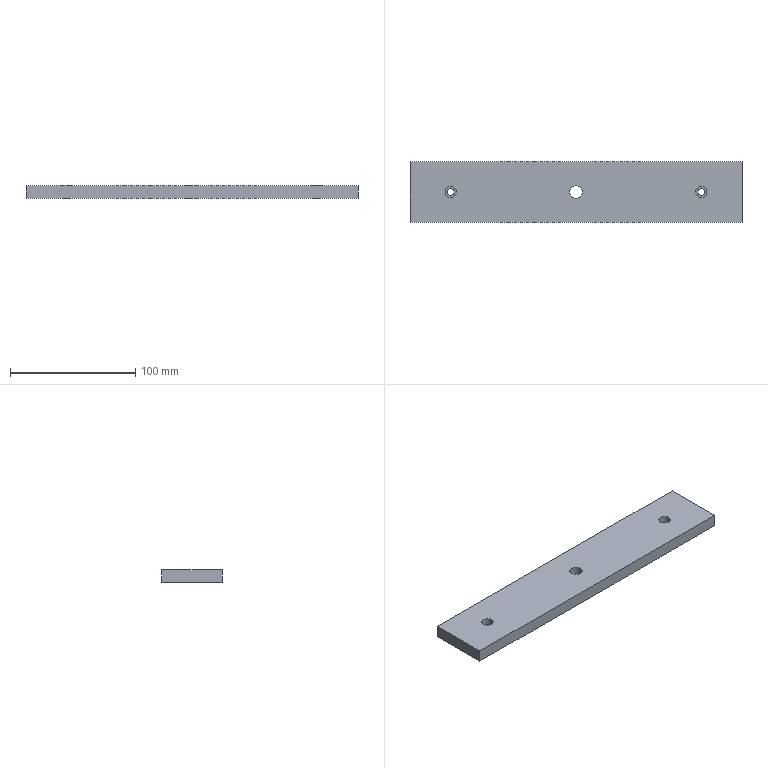Part | STEP file | B1-008 | 1 solid | 18 faces | box 265 x 48 x 10 mm | volume 125461 mm3 | cylinder 10 | plane 8 | commonest cylinder face diameters 5.5 x4 9 x4 10 x2
STEP:
#1=CARTESIAN_POINT('',(0.,0.,0.));
#2=DIRECTION('',(0.,0.,1.));
#3=DIRECTION('',(1.,0.,0.));
#4=AXIS2_PLACEMENT_3D('',#1,#2,#3);
#5=CARTESIAN_POINT('',(-95.5,0.,-1.));
#6=VERTEX_POINT('',#5);
#7=CARTESIAN_POINT('',(-95.5,0.,5.));
#8=VERTEX_POINT('',#7);
#9=CARTESIAN_POINT('',(-95.5,0.,-1.));
#10=DIRECTION('',(0.,0.,1.));
#11=VECTOR('',#10,1.);
#12=LINE('',#9,#11);
#13=CARTESIAN_POINT('',(-100.,0.,-1.));
#14=DIRECTION('',(0.,0.,1.));
#15=DIRECTION('',(1.,0.,0.));
#16=AXIS2_PLACEMENT_3D('',#13,#14,#15);
#17=CYLINDRICAL_SURFACE('',#16,4.5);
#18=CARTESIAN_POINT('',(6.283,0.));
#19=DIRECTION('',(0.,1.));
#20=VECTOR('',#19,1.);
#21=LINE('',#18,#20);
#22=(GEOMETRIC_REPRESENTATION_CONTEXT(2)PARAMETRIC_REPRESENTATION_CONTEXT()REPRESENTATION_CONTEXT('',''));
#23=DEFINITIONAL_REPRESENTATION('',(#21),#22);
#24=PCURVE('',#17,#23);
#25=CARTESIAN_POINT('',(-100.,0.,-1.));
#26=DIRECTION('',(0.,0.,1.));
#27=DIRECTION('',(1.,0.,0.));
#28=AXIS2_PLACEMENT_3D('',#25,#26,#27);
#29=CYLINDRICAL_SURFACE('',#28,4.5);
#30=CARTESIAN_POINT('',(0.,0.));
#31=DIRECTION('',(0.,1.));
#32=VECTOR('',#31,1.);
#33=LINE('',#30,#32);
#34=(GEOMETRIC_REPRESENTATION_CONTEXT(2)PARAMETRIC_REPRESENTATION_CONTEXT()REPRESENTATION_CONTEXT('',''));
#35=DEFINITIONAL_REPRESENTATION('',(#33),#34);
#36=PCURVE('',#29,#35);
#37=SURFACE_CURVE('',#12,(#24,#36),.PCURVE_S1.);
#38=EDGE_CURVE('',#6,#8,#37,.T.);
#39=ORIENTED_EDGE('',*,*,#38,.T.);
#40=CARTESIAN_POINT('',(-104.5,0.,5.));
#41=VERTEX_POINT('',#40);
#42=CARTESIAN_POINT('',(-100.,0.,5.));
#43=DIRECTION('',(0.,0.,1.));
#44=DIRECTION('',(1.,0.,0.));
#45=AXIS2_PLACEMENT_3D('',#42,#43,#44);
#46=CIRCLE('',#45,4.5);
#47=CARTESIAN_POINT('',(0.,6.));
#48=DIRECTION('',(1.,0.));
#49=VECTOR('',#48,1.);
#50=LINE('',#47,#49);
#51=(GEOMETRIC_REPRESENTATION_CONTEXT(2)PARAMETRIC_REPRESENTATION_CONTEXT()REPRESENTATION_CONTEXT('',''));
#52=DEFINITIONAL_REPRESENTATION('',(#50),#51);
#53=PCURVE('',#17,#52);
#54=CARTESIAN_POINT('',(0.,0.,5.));
#55=DIRECTION('',(0.,0.,1.));
#56=DIRECTION('',(1.,0.,0.));
#57=AXIS2_PLACEMENT_3D('',#54,#55,#56);
#58=PLANE('',#57);
#59=CARTESIAN_POINT('',(-100.,0.));
#60=DIRECTION('',(1.,0.));
#61=AXIS2_PLACEMENT_2D('',#59,#60);
#62=CIRCLE('',#61,4.5);
#63=(GEOMETRIC_REPRESENTATION_CONTEXT(2)PARAMETRIC_REPRESENTATION_CONTEXT()REPRESENTATION_CONTEXT('',''));
#64=DEFINITIONAL_REPRESENTATION('',(#62),#63);
#65=PCURVE('',#58,#64);
#66=SURFACE_CURVE('',#46,(#53,#65),.PCURVE_S1.);
#67=EDGE_CURVE('',#41,#8,#66,.T.);
#68=ORIENTED_EDGE('',*,*,#67,.F.);
#69=CARTESIAN_POINT('',(-104.5,0.,-1.));
#70=VERTEX_POINT('',#69);
#71=CARTESIAN_POINT('',(-104.5,0.,-1.));
#72=DIRECTION('',(0.,0.,1.));
#73=VECTOR('',#72,1.);
#74=LINE('',#71,#73);
#75=CARTESIAN_POINT('',(3.142,0.));
#76=DIRECTION('',(0.,1.));
#77=VECTOR('',#76,1.);
#78=LINE('',#75,#77);
#79=(GEOMETRIC_REPRESENTATION_CONTEXT(2)PARAMETRIC_REPRESENTATION_CONTEXT()REPRESENTATION_CONTEXT('',''));
#80=DEFINITIONAL_REPRESENTATION('',(#78),#79);
#81=PCURVE('',#17,#80);
#82=CARTESIAN_POINT('',(3.142,0.));
#83=DIRECTION('',(0.,1.));
#84=VECTOR('',#83,1.);
#85=LINE('',#82,#84);
#86=(GEOMETRIC_REPRESENTATION_CONTEXT(2)PARAMETRIC_REPRESENTATION_CONTEXT()REPRESENTATION_CONTEXT('',''));
#87=DEFINITIONAL_REPRESENTATION('',(#85),#86);
#88=PCURVE('',#29,#87);
#89=SURFACE_CURVE('',#74,(#81,#88),.PCURVE_S1.);
#90=EDGE_CURVE('',#70,#41,#89,.T.);
#91=ORIENTED_EDGE('',*,*,#90,.F.);
#92=CARTESIAN_POINT('',(-100.,0.,-1.));
#93=DIRECTION('',(0.,0.,1.));
#94=DIRECTION('',(1.,0.,0.));
#95=AXIS2_PLACEMENT_3D('',#92,#93,#94);
#96=CIRCLE('',#95,4.5);
#97=CARTESIAN_POINT('',(0.,0.));
#98=DIRECTION('',(1.,0.));
#99=VECTOR('',#98,1.);
#100=LINE('',#97,#99);
#101=(GEOMETRIC_REPRESENTATION_CONTEXT(2)PARAMETRIC_REPRESENTATION_CONTEXT()REPRESENTATION_CONTEXT('',''));
#102=DEFINITIONAL_REPRESENTATION('',(#100),#101);
#103=PCURVE('',#17,#102);
#104=CARTESIAN_POINT('',(-100.,0.,-1.));
#105=DIRECTION('',(0.,0.,1.));
#106=DIRECTION('',(1.,0.,0.));
#107=AXIS2_PLACEMENT_3D('',#104,#105,#106);
#108=PLANE('',#107);
#109=CARTESIAN_POINT('',(0.,0.));
#110=DIRECTION('',(1.,0.));
#111=AXIS2_PLACEMENT_2D('',#109,#110);
#112=CIRCLE('',#111,4.5);
#113=(GEOMETRIC_REPRESENTATION_CONTEXT(2)PARAMETRIC_REPRESENTATION_CONTEXT()REPRESENTATION_CONTEXT('',''));
#114=DEFINITIONAL_REPRESENTATION('',(#112),#113);
#115=PCURVE('',#108,#114);
#116=SURFACE_CURVE('',#96,(#103,#115),.PCURVE_S1.);
#117=EDGE_CURVE('',#70,#6,#116,.T.);
#118=ORIENTED_EDGE('',*,*,#117,.T.);
#119=EDGE_LOOP('',(#39,#68,#91,#118));
#120=FACE_BOUND('',#119,.F.);
#121=ADVANCED_FACE('',(#120),#17,.F.);
#122=CARTESIAN_POINT('',(104.5,0.,-1.));
#123=VERTEX_POINT('',#122);
#124=CARTESIAN_POINT('',(104.5,0.,5.));
#125=VERTEX_POINT('',#124);
#126=CARTESIAN_POINT('',(104.5,0.,-1.));
#127=DIRECTION('',(0.,0.,1.));
#128=VECTOR('',#127,1.);
#129=LINE('',#126,#128);
#130=CARTESIAN_POINT('',(100.,0.,-1.));
#131=DIRECTION('',(0.,0.,1.));
#132=DIRECTION('',(1.,0.,0.));
#133=AXIS2_PLACEMENT_3D('',#130,#131,#132);
#134=CYLINDRICAL_SURFACE('',#133,4.5);
#135=CARTESIAN_POINT('',(6.283,0.));
#136=DIRECTION('',(0.,1.));
#137=VECTOR('',#136,1.);
#138=LINE('',#135,#137);
#139=(GEOMETRIC_REPRESENTATION_CONTEXT(2)PARAMETRIC_REPRESENTATION_CONTEXT()REPRESENTATION_CONTEXT('',''));
#140=DEFINITIONAL_REPRESENTATION('',(#138),#139);
#141=PCURVE('',#134,#140);
#142=CARTESIAN_POINT('',(100.,0.,-1.));
#143=DIRECTION('',(0.,0.,1.));
#144=DIRECTION('',(1.,0.,0.));
#145=AXIS2_PLACEMENT_3D('',#142,#143,#144);
#146=CYLINDRICAL_SURFACE('',#145,4.5);
#147=CARTESIAN_POINT('',(0.,0.));
#148=DIRECTION('',(0.,1.));
#149=VECTOR('',#148,1.);
#150=LINE('',#147,#149);
#151=(GEOMETRIC_REPRESENTATION_CONTEXT(2)PARAMETRIC_REPRESENTATION_CONTEXT()REPRESENTATION_CONTEXT('',''));
#152=DEFINITIONAL_REPRESENTATION('',(#150),#151);
#153=PCURVE('',#146,#152);
#154=SURFACE_CURVE('',#129,(#141,#153),.PCURVE_S1.);
#155=EDGE_CURVE('',#123,#125,#154,.T.);
#156=ORIENTED_EDGE('',*,*,#155,.T.);
#157=CARTESIAN_POINT('',(95.5,0.,5.));
#158=VERTEX_POINT('',#157);
#159=CARTESIAN_POINT('',(100.,0.,5.));
#160=DIRECTION('',(0.,0.,1.));
#161=DIRECTION('',(1.,0.,0.));
#162=AXIS2_PLACEMENT_3D('',#159,#160,#161);
#163=CIRCLE('',#162,4.5);
#164=CARTESIAN_POINT('',(0.,6.));
#165=DIRECTION('',(1.,0.));
#166=VECTOR('',#165,1.);
#167=LINE('',#164,#166);
#168=(GEOMETRIC_REPRESENTATION_CONTEXT(2)PARAMETRIC_REPRESENTATION_CONTEXT()REPRESENTATION_CONTEXT('',''));
#169=DEFINITIONAL_REPRESENTATION('',(#167),#168);
#170=PCURVE('',#134,#169);
#171=CARTESIAN_POINT('',(100.,0.));
#172=DIRECTION('',(1.,0.));
#173=AXIS2_PLACEMENT_2D('',#171,#172);
#174=CIRCLE('',#173,4.5);
#175=(GEOMETRIC_REPRESENTATION_CONTEXT(2)PARAMETRIC_REPRESENTATION_CONTEXT()REPRESENTATION_CONTEXT('',''));
#176=DEFINITIONAL_REPRESENTATION('',(#174),#175);
#177=PCURVE('',#58,#176);
#178=SURFACE_CURVE('',#163,(#170,#177),.PCURVE_S1.);
#179=EDGE_CURVE('',#158,#125,#178,.T.);
#180=ORIENTED_EDGE('',*,*,#179,.F.);
#181=CARTESIAN_POINT('',(95.5,0.,-1.));
#182=VERTEX_POINT('',#181);
#183=CARTESIAN_POINT('',(95.5,0.,-1.));
#184=DIRECTION('',(0.,0.,1.));
#185=VECTOR('',#184,1.);
#186=LINE('',#183,#185);
#187=CARTESIAN_POINT('',(3.142,0.));
#188=DIRECTION('',(0.,1.));
#189=VECTOR('',#188,1.);
#190=LINE('',#187,#189);
#191=(GEOMETRIC_REPRESENTATION_CONTEXT(2)PARAMETRIC_REPRESENTATION_CONTEXT()REPRESENTATION_CONTEXT('',''));
#192=DEFINITIONAL_REPRESENTATION('',(#190),#191);
#193=PCURVE('',#134,#192);
#194=CARTESIAN_POINT('',(3.142,0.));
#195=DIRECTION('',(0.,1.));
#196=VECTOR('',#195,1.);
#197=LINE('',#194,#196);
#198=(GEOMETRIC_REPRESENTATION_CONTEXT(2)PARAMETRIC_REPRESENTATION_CONTEXT()REPRESENTATION_CONTEXT('',''));
#199=DEFINITIONAL_REPRESENTATION('',(#197),#198);
#200=PCURVE('',#146,#199);
#201=SURFACE_CURVE('',#186,(#193,#200),.PCURVE_S1.);
#202=EDGE_CURVE('',#182,#158,#201,.T.);
#203=ORIENTED_EDGE('',*,*,#202,.F.);
#204=CARTESIAN_POINT('',(100.,0.,-1.));
#205=DIRECTION('',(0.,0.,1.));
#206=DIRECTION('',(1.,0.,0.));
#207=AXIS2_PLACEMENT_3D('',#204,#205,#206);
#208=CIRCLE('',#207,4.5);
#209=CARTESIAN_POINT('',(0.,0.));
#210=DIRECTION('',(1.,0.));
#211=VECTOR('',#210,1.);
#212=LINE('',#209,#211);
#213=(GEOMETRIC_REPRESENTATION_CONTEXT(2)PARAMETRIC_REPRESENTATION_CONTEXT()REPRESENTATION_CONTEXT('',''));
#214=DEFINITIONAL_REPRESENTATION('',(#212),#213);
#215=PCURVE('',#134,#214);
#216=CARTESIAN_POINT('',(100.,0.,-1.));
#217=DIRECTION('',(0.,0.,1.));
#218=DIRECTION('',(1.,0.,0.));
#219=AXIS2_PLACEMENT_3D('',#216,#217,#218);
#220=PLANE('',#219);
#221=CARTESIAN_POINT('',(0.,0.));
#222=DIRECTION('',(1.,0.));
#223=AXIS2_PLACEMENT_2D('',#221,#222);
#224=CIRCLE('',#223,4.5);
#225=(GEOMETRIC_REPRESENTATION_CONTEXT(2)PARAMETRIC_REPRESENTATION_CONTEXT()REPRESENTATION_CONTEXT('',''));
#226=DEFINITIONAL_REPRESENTATION('',(#224),#225);
#227=PCURVE('',#220,#226);
#228=SURFACE_CURVE('',#208,(#215,#227),.PCURVE_S1.);
#229=EDGE_CURVE('',#182,#123,#228,.T.);
#230=ORIENTED_EDGE('',*,*,#229,.T.);
#231=EDGE_LOOP('',(#156,#180,#203,#230));
#232=FACE_BOUND('',#231,.F.);
#233=ADVANCED_FACE('',(#232),#134,.F.);
#234=CARTESIAN_POINT('',(5.,0.,-5.));
#235=VERTEX_POINT('',#234);
#236=CARTESIAN_POINT('',(5.,0.,5.));
#237=VERTEX_POINT('',#236);
#238=CARTESIAN_POINT('',(5.,0.,-19.142));
#239=DIRECTION('',(0.,0.,1.));
#240=VECTOR('',#239,1.);
#241=LINE('',#238,#240);
#242=CARTESIAN_POINT('',(0.,0.,-19.142));
#243=DIRECTION('',(0.,0.,1.));
#244=DIRECTION('',(1.,0.,0.));
#245=AXIS2_PLACEMENT_3D('',#242,#243,#244);
#246=CYLINDRICAL_SURFACE('',#245,5.);
#247=CARTESIAN_POINT('',(6.283,0.));
#248=DIRECTION('',(0.,1.));
#249=VECTOR('',#248,1.);
#250=LINE('',#247,#249);
#251=(GEOMETRIC_REPRESENTATION_CONTEXT(2)PARAMETRIC_REPRESENTATION_CONTEXT()REPRESENTATION_CONTEXT('',''));
#252=DEFINITIONAL_REPRESENTATION('',(#250),#251);
#253=PCURVE('',#246,#252);
#254=CARTESIAN_POINT('',(0.,0.,-19.142));
#255=DIRECTION('',(0.,0.,1.));
#256=DIRECTION('',(1.,0.,0.));
#257=AXIS2_PLACEMENT_3D('',#254,#255,#256);
#258=CYLINDRICAL_SURFACE('',#257,5.);
#259=CARTESIAN_POINT('',(0.,0.));
#260=DIRECTION('',(0.,1.));
#261=VECTOR('',#260,1.);
#262=LINE('',#259,#261);
#263=(GEOMETRIC_REPRESENTATION_CONTEXT(2)PARAMETRIC_REPRESENTATION_CONTEXT()REPRESENTATION_CONTEXT('',''));
#264=DEFINITIONAL_REPRESENTATION('',(#262),#263);
#265=PCURVE('',#258,#264);
#266=SURFACE_CURVE('',#241,(#253,#265),.PCURVE_S1.);
#267=EDGE_CURVE('',#235,#237,#266,.T.);
#268=ORIENTED_EDGE('',*,*,#267,.T.);
#269=CARTESIAN_POINT('',(-5.,0.,5.));
#270=VERTEX_POINT('',#269);
#271=CARTESIAN_POINT('',(0.,0.,5.));
#272=DIRECTION('',(0.,0.,1.));
#273=DIRECTION('',(1.,0.,0.));
#274=AXIS2_PLACEMENT_3D('',#271,#272,#273);
#275=CIRCLE('',#274,5.);
#276=CARTESIAN_POINT('',(0.,24.142));
#277=DIRECTION('',(1.,0.));
#278=VECTOR('',#277,1.);
#279=LINE('',#276,#278);
#280=(GEOMETRIC_REPRESENTATION_CONTEXT(2)PARAMETRIC_REPRESENTATION_CONTEXT()REPRESENTATION_CONTEXT('',''));
#281=DEFINITIONAL_REPRESENTATION('',(#279),#280);
#282=PCURVE('',#246,#281);
#283=CARTESIAN_POINT('',(0.,0.));
#284=DIRECTION('',(1.,0.));
#285=AXIS2_PLACEMENT_2D('',#283,#284);
#286=CIRCLE('',#285,5.);
#287=(GEOMETRIC_REPRESENTATION_CONTEXT(2)PARAMETRIC_REPRESENTATION_CONTEXT()REPRESENTATION_CONTEXT('',''));
#288=DEFINITIONAL_REPRESENTATION('',(#286),#287);
#289=PCURVE('',#58,#288);
#290=SURFACE_CURVE('',#275,(#282,#289),.PCURVE_S1.);
#291=EDGE_CURVE('',#270,#237,#290,.T.);
#292=ORIENTED_EDGE('',*,*,#291,.F.);
#293=CARTESIAN_POINT('',(-5.,0.,-5.));
#294=VERTEX_POINT('',#293);
#295=CARTESIAN_POINT('',(-5.,0.,-19.142));
#296=DIRECTION('',(0.,0.,1.));
#297=VECTOR('',#296,1.);
#298=LINE('',#295,#297);
#299=CARTESIAN_POINT('',(3.142,0.));
#300=DIRECTION('',(0.,1.));
#301=VECTOR('',#300,1.);
#302=LINE('',#299,#301);
#303=(GEOMETRIC_REPRESENTATION_CONTEXT(2)PARAMETRIC_REPRESENTATION_CONTEXT()REPRESENTATION_CONTEXT('',''));
#304=DEFINITIONAL_REPRESENTATION('',(#302),#303);
#305=PCURVE('',#246,#304);
#306=CARTESIAN_POINT('',(3.142,0.));
#307=DIRECTION('',(0.,1.));
#308=VECTOR('',#307,1.);
#309=LINE('',#306,#308);
#310=(GEOMETRIC_REPRESENTATION_CONTEXT(2)PARAMETRIC_REPRESENTATION_CONTEXT()REPRESENTATION_CONTEXT('',''));
#311=DEFINITIONAL_REPRESENTATION('',(#309),#310);
#312=PCURVE('',#258,#311);
#313=SURFACE_CURVE('',#298,(#305,#312),.PCURVE_S1.);
#314=EDGE_CURVE('',#294,#270,#313,.T.);
#315=ORIENTED_EDGE('',*,*,#314,.F.);
#316=CARTESIAN_POINT('',(0.,0.,-5.));
#317=DIRECTION('',(0.,0.,-1.));
#318=DIRECTION('',(1.,0.,0.));
#319=AXIS2_PLACEMENT_3D('',#316,#317,#318);
#320=CIRCLE('',#319,5.);
#321=CARTESIAN_POINT('',(6.283,14.142));
#322=DIRECTION('',(-1.,0.));
#323=VECTOR('',#322,1.);
#324=LINE('',#321,#323);
#325=(GEOMETRIC_REPRESENTATION_CONTEXT(2)PARAMETRIC_REPRESENTATION_CONTEXT()REPRESENTATION_CONTEXT('',''));
#326=DEFINITIONAL_REPRESENTATION('',(#324),#325);
#327=PCURVE('',#246,#326);
#328=CARTESIAN_POINT('',(0.,0.,-5.));
#329=DIRECTION('',(0.,0.,1.));
#330=DIRECTION('',(1.,0.,0.));
#331=AXIS2_PLACEMENT_3D('',#328,#329,#330);
#332=PLANE('',#331);
#333=CARTESIAN_POINT('',(5.,0.));
#334=CARTESIAN_POINT('',(5.,-8.66));
#335=CARTESIAN_POINT('',(-2.5,-4.33));
#336=CARTESIAN_POINT('',(-10.,0.));
#337=CARTESIAN_POINT('',(-2.5,4.33));
#338=CARTESIAN_POINT('',(5.,8.66));
#339=CARTESIAN_POINT('',(5.,0.));
#340=(BOUNDED_CURVE()B_SPLINE_CURVE(2,(#333,#334,#335,#336,#337,#338,#339),.UNSPECIFIED.,.T.,.F.)B_SPLINE_CURVE_WITH_KNOTS((1,2,2,2,2,1),(-2.094,0.,2.094,4.189,6.283,8.378),.UNSPECIFIED.)CURVE()GEOMETRIC_REPRESENTATION_ITEM()RATIONAL_B_SPLINE_CURVE((1.,0.5,1.,0.5,1.,0.5,1.))REPRESENTATION_ITEM(''));
#341=(GEOMETRIC_REPRESENTATION_CONTEXT(2)PARAMETRIC_REPRESENTATION_CONTEXT()REPRESENTATION_CONTEXT('',''));
#342=DEFINITIONAL_REPRESENTATION('',(#340),#341);
#343=PCURVE('',#332,#342);
#344=SURFACE_CURVE('',#320,(#327,#343),.PCURVE_S1.);
#345=EDGE_CURVE('',#235,#294,#344,.T.);
#346=ORIENTED_EDGE('',*,*,#345,.F.);
#347=EDGE_LOOP('',(#268,#292,#315,#346));
#348=FACE_BOUND('',#347,.F.);
#349=ADVANCED_FACE('',(#348),#246,.F.);
#350=CARTESIAN_POINT('',(97.25,0.,-1.));
#351=VERTEX_POINT('',#350);
#352=CARTESIAN_POINT('',(97.25,0.,-5.));
#353=VERTEX_POINT('',#352);
#354=CARTESIAN_POINT('',(97.25,0.,12.778));
#355=DIRECTION('',(0.,0.,-1.));
#356=VECTOR('',#355,1.);
#357=LINE('',#354,#356);
#358=CARTESIAN_POINT('',(100.,0.,12.778));
#359=DIRECTION('',(0.,0.,-1.));
#360=DIRECTION('',(-1.,0.,0.));
#361=AXIS2_PLACEMENT_3D('',#358,#359,#360);
#362=CYLINDRICAL_SURFACE('',#361,2.75);
#363=CARTESIAN_POINT('',(6.283,0.));
#364=DIRECTION('',(0.,1.));
#365=VECTOR('',#364,1.);
#366=LINE('',#363,#365);
#367=(GEOMETRIC_REPRESENTATION_CONTEXT(2)PARAMETRIC_REPRESENTATION_CONTEXT()REPRESENTATION_CONTEXT('',''));
#368=DEFINITIONAL_REPRESENTATION('',(#366),#367);
#369=PCURVE('',#362,#368);
#370=CARTESIAN_POINT('',(100.,0.,12.778));
#371=DIRECTION('',(0.,0.,-1.));
#372=DIRECTION('',(-1.,0.,0.));
#373=AXIS2_PLACEMENT_3D('',#370,#371,#372);
#374=CYLINDRICAL_SURFACE('',#373,2.75);
#375=CARTESIAN_POINT('',(0.,0.));
#376=DIRECTION('',(0.,1.));
#377=VECTOR('',#376,1.);
#378=LINE('',#375,#377);
#379=(GEOMETRIC_REPRESENTATION_CONTEXT(2)PARAMETRIC_REPRESENTATION_CONTEXT()REPRESENTATION_CONTEXT('',''));
#380=DEFINITIONAL_REPRESENTATION('',(#378),#379);
#381=PCURVE('',#374,#380);
#382=SURFACE_CURVE('',#357,(#369,#381),.PCURVE_S1.);
#383=EDGE_CURVE('',#351,#353,#382,.T.);
#384=ORIENTED_EDGE('',*,*,#383,.T.);
#385=CARTESIAN_POINT('',(102.75,0.,-5.));
#386=VERTEX_POINT('',#385);
#387=CARTESIAN_POINT('',(100.,0.,-5.));
#388=DIRECTION('',(0.,0.,-1.));
#389=DIRECTION('',(-1.,0.,0.));
#390=AXIS2_PLACEMENT_3D('',#387,#388,#389);
#391=CIRCLE('',#390,2.75);
#392=CARTESIAN_POINT('',(0.,17.778));
#393=DIRECTION('',(1.,0.));
#394=VECTOR('',#393,1.);
#395=LINE('',#392,#394);
#396=(GEOMETRIC_REPRESENTATION_CONTEXT(2)PARAMETRIC_REPRESENTATION_CONTEXT()REPRESENTATION_CONTEXT('',''));
#397=DEFINITIONAL_REPRESENTATION('',(#395),#396);
#398=PCURVE('',#362,#397);
#399=CARTESIAN_POINT('',(97.25,0.));
#400=CARTESIAN_POINT('',(97.25,4.763));
#401=CARTESIAN_POINT('',(101.375,2.382));
#402=CARTESIAN_POINT('',(105.5,0.));
#403=CARTESIAN_POINT('',(101.375,-2.382));
#404=CARTESIAN_POINT('',(97.25,-4.763));
#405=CARTESIAN_POINT('',(97.25,0.));
#406=(BOUNDED_CURVE()B_SPLINE_CURVE(2,(#399,#400,#401,#402,#403,#404,#405),.UNSPECIFIED.,.T.,.F.)B_SPLINE_CURVE_WITH_KNOTS((1,2,2,2,2,1),(-2.094,0.,2.094,4.189,6.283,8.378),.UNSPECIFIED.)CURVE()GEOMETRIC_REPRESENTATION_ITEM()RATIONAL_B_SPLINE_CURVE((1.,0.5,1.,0.5,1.,0.5,1.))REPRESENTATION_ITEM(''));
#407=(GEOMETRIC_REPRESENTATION_CONTEXT(2)PARAMETRIC_REPRESENTATION_CONTEXT()REPRESENTATION_CONTEXT('',''));
#408=DEFINITIONAL_REPRESENTATION('',(#406),#407);
#409=PCURVE('',#332,#408);
#410=SURFACE_CURVE('',#391,(#398,#409),.PCURVE_S1.);
#411=EDGE_CURVE('',#386,#353,#410,.T.);
#412=ORIENTED_EDGE('',*,*,#411,.F.);
#413=CARTESIAN_POINT('',(102.75,0.,-1.));
#414=VERTEX_POINT('',#413);
#415=CARTESIAN_POINT('',(102.75,0.,12.778));
#416=DIRECTION('',(0.,0.,-1.));
#417=VECTOR('',#416,1.);
#418=LINE('',#415,#417);
#419=CARTESIAN_POINT('',(3.142,0.));
#420=DIRECTION('',(0.,1.));
#421=VECTOR('',#420,1.);
#422=LINE('',#419,#421);
#423=(GEOMETRIC_REPRESENTATION_CONTEXT(2)PARAMETRIC_REPRESENTATION_CONTEXT()REPRESENTATION_CONTEXT('',''));
#424=DEFINITIONAL_REPRESENTATION('',(#422),#423);
#425=PCURVE('',#362,#424);
#426=CARTESIAN_POINT('',(3.142,0.));
#427=DIRECTION('',(0.,1.));
#428=VECTOR('',#427,1.);
#429=LINE('',#426,#428);
#430=(GEOMETRIC_REPRESENTATION_CONTEXT(2)PARAMETRIC_REPRESENTATION_CONTEXT()REPRESENTATION_CONTEXT('',''));
#431=DEFINITIONAL_REPRESENTATION('',(#429),#430);
#432=PCURVE('',#374,#431);
#433=SURFACE_CURVE('',#418,(#425,#432),.PCURVE_S1.);
#434=EDGE_CURVE('',#414,#386,#433,.T.);
#435=ORIENTED_EDGE('',*,*,#434,.F.);
#436=CARTESIAN_POINT('',(100.,0.,-1.));
#437=DIRECTION('',(0.,0.,-1.));
#438=DIRECTION('',(1.,0.,0.));
#439=AXIS2_PLACEMENT_3D('',#436,#437,#438);
#440=CIRCLE('',#439,2.75);
#441=CARTESIAN_POINT('',(3.142,13.778));
#442=DIRECTION('',(1.,0.));
#443=VECTOR('',#442,1.);
#444=LINE('',#441,#443);
#445=(GEOMETRIC_REPRESENTATION_CONTEXT(2)PARAMETRIC_REPRESENTATION_CONTEXT()REPRESENTATION_CONTEXT('',''));
#446=DEFINITIONAL_REPRESENTATION('',(#444),#445);
#447=PCURVE('',#362,#446);
#448=CARTESIAN_POINT('',(2.75,0.));
#449=CARTESIAN_POINT('',(2.75,-4.763));
#450=CARTESIAN_POINT('',(-1.375,-2.382));
#451=CARTESIAN_POINT('',(-5.5,0.));
#452=CARTESIAN_POINT('',(-1.375,2.382));
#453=CARTESIAN_POINT('',(2.75,4.763));
#454=CARTESIAN_POINT('',(2.75,0.));
#455=(BOUNDED_CURVE()B_SPLINE_CURVE(2,(#448,#449,#450,#451,#452,#453,#454),.UNSPECIFIED.,.T.,.F.)B_SPLINE_CURVE_WITH_KNOTS((1,2,2,2,2,1),(-2.094,0.,2.094,4.189,6.283,8.378),.UNSPECIFIED.)CURVE()GEOMETRIC_REPRESENTATION_ITEM()RATIONAL_B_SPLINE_CURVE((1.,0.5,1.,0.5,1.,0.5,1.))REPRESENTATION_ITEM(''));
#456=(GEOMETRIC_REPRESENTATION_CONTEXT(2)PARAMETRIC_REPRESENTATION_CONTEXT()REPRESENTATION_CONTEXT('',''));
#457=DEFINITIONAL_REPRESENTATION('',(#455),#456);
#458=PCURVE('',#220,#457);
#459=SURFACE_CURVE('',#440,(#447,#458),.PCURVE_S1.);
#460=EDGE_CURVE('',#414,#351,#459,.T.);
#461=ORIENTED_EDGE('',*,*,#460,.T.);
#462=EDGE_LOOP('',(#384,#412,#435,#461));
#463=FACE_BOUND('',#462,.F.);
#464=ADVANCED_FACE('',(#463),#362,.F.);
#465=CARTESIAN_POINT('',(-102.75,0.,-1.));
#466=VERTEX_POINT('',#465);
#467=CARTESIAN_POINT('',(-102.75,0.,-5.));
#468=VERTEX_POINT('',#467);
#469=CARTESIAN_POINT('',(-102.75,0.,12.778));
#470=DIRECTION('',(0.,0.,-1.));
#471=VECTOR('',#470,1.);
#472=LINE('',#469,#471);
#473=CARTESIAN_POINT('',(-100.,0.,12.778));
#474=DIRECTION('',(0.,0.,-1.));
#475=DIRECTION('',(-1.,0.,0.));
#476=AXIS2_PLACEMENT_3D('',#473,#474,#475);
#477=CYLINDRICAL_SURFACE('',#476,2.75);
#478=CARTESIAN_POINT('',(6.283,0.));
#479=DIRECTION('',(0.,1.));
#480=VECTOR('',#479,1.);
#481=LINE('',#478,#480);
#482=(GEOMETRIC_REPRESENTATION_CONTEXT(2)PARAMETRIC_REPRESENTATION_CONTEXT()REPRESENTATION_CONTEXT('',''));
#483=DEFINITIONAL_REPRESENTATION('',(#481),#482);
#484=PCURVE('',#477,#483);
#485=CARTESIAN_POINT('',(-100.,0.,12.778));
#486=DIRECTION('',(0.,0.,-1.));
#487=DIRECTION('',(-1.,0.,0.));
#488=AXIS2_PLACEMENT_3D('',#485,#486,#487);
#489=CYLINDRICAL_SURFACE('',#488,2.75);
#490=CARTESIAN_POINT('',(0.,0.));
#491=DIRECTION('',(0.,1.));
#492=VECTOR('',#491,1.);
#493=LINE('',#490,#492);
#494=(GEOMETRIC_REPRESENTATION_CONTEXT(2)PARAMETRIC_REPRESENTATION_CONTEXT()REPRESENTATION_CONTEXT('',''));
#495=DEFINITIONAL_REPRESENTATION('',(#493),#494);
#496=PCURVE('',#489,#495);
#497=SURFACE_CURVE('',#472,(#484,#496),.PCURVE_S1.);
#498=EDGE_CURVE('',#466,#468,#497,.T.);
#499=ORIENTED_EDGE('',*,*,#498,.T.);
#500=CARTESIAN_POINT('',(-97.25,0.,-5.));
#501=VERTEX_POINT('',#500);
#502=CARTESIAN_POINT('',(-100.,0.,-5.));
#503=DIRECTION('',(0.,0.,-1.));
#504=DIRECTION('',(-1.,0.,0.));
#505=AXIS2_PLACEMENT_3D('',#502,#503,#504);
#506=CIRCLE('',#505,2.75);
#507=CARTESIAN_POINT('',(0.,17.778));
#508=DIRECTION('',(1.,0.));
#509=VECTOR('',#508,1.);
#510=LINE('',#507,#509);
#511=(GEOMETRIC_REPRESENTATION_CONTEXT(2)PARAMETRIC_REPRESENTATION_CONTEXT()REPRESENTATION_CONTEXT('',''));
#512=DEFINITIONAL_REPRESENTATION('',(#510),#511);
#513=PCURVE('',#477,#512);
#514=CARTESIAN_POINT('',(-102.75,0.));
#515=CARTESIAN_POINT('',(-102.75,4.763));
#516=CARTESIAN_POINT('',(-98.625,2.382));
#517=CARTESIAN_POINT('',(-94.5,0.));
#518=CARTESIAN_POINT('',(-98.625,-2.382));
#519=CARTESIAN_POINT('',(-102.75,-4.763));
#520=CARTESIAN_POINT('',(-102.75,0.));
#521=(BOUNDED_CURVE()B_SPLINE_CURVE(2,(#514,#515,#516,#517,#518,#519,#520),.UNSPECIFIED.,.T.,.F.)B_SPLINE_CURVE_WITH_KNOTS((1,2,2,2,2,1),(-2.094,0.,2.094,4.189,6.283,8.378),.UNSPECIFIED.)CURVE()GEOMETRIC_REPRESENTATION_ITEM()RATIONAL_B_SPLINE_CURVE((1.,0.5,1.,0.5,1.,0.5,1.))REPRESENTATION_ITEM(''));
#522=(GEOMETRIC_REPRESENTATION_CONTEXT(2)PARAMETRIC_REPRESENTATION_CONTEXT()REPRESENTATION_CONTEXT('',''));
#523=DEFINITIONAL_REPRESENTATION('',(#521),#522);
#524=PCURVE('',#332,#523);
#525=SURFACE_CURVE('',#506,(#513,#524),.PCURVE_S1.);
#526=EDGE_CURVE('',#501,#468,#525,.T.);
#527=ORIENTED_EDGE('',*,*,#526,.F.);
#528=CARTESIAN_POINT('',(-97.25,0.,-1.));
#529=VERTEX_POINT('',#528);
#530=CARTESIAN_POINT('',(-97.25,0.,12.778));
#531=DIRECTION('',(0.,0.,-1.));
#532=VECTOR('',#531,1.);
#533=LINE('',#530,#532);
#534=CARTESIAN_POINT('',(3.142,0.));
#535=DIRECTION('',(0.,1.));
#536=VECTOR('',#535,1.);
#537=LINE('',#534,#536);
#538=(GEOMETRIC_REPRESENTATION_CONTEXT(2)PARAMETRIC_REPRESENTATION_CONTEXT()REPRESENTATION_CONTEXT('',''));
#539=DEFINITIONAL_REPRESENTATION('',(#537),#538);
#540=PCURVE('',#477,#539);
#541=CARTESIAN_POINT('',(3.142,0.));
#542=DIRECTION('',(0.,1.));
#543=VECTOR('',#542,1.);
#544=LINE('',#541,#543);
#545=(GEOMETRIC_REPRESENTATION_CONTEXT(2)PARAMETRIC_REPRESENTATION_CONTEXT()REPRESENTATION_CONTEXT('',''));
#546=DEFINITIONAL_REPRESENTATION('',(#544),#545);
#547=PCURVE('',#489,#546);
#548=SURFACE_CURVE('',#533,(#540,#547),.PCURVE_S1.);
#549=EDGE_CURVE('',#529,#501,#548,.T.);
#550=ORIENTED_EDGE('',*,*,#549,.F.);
#551=CARTESIAN_POINT('',(-100.,0.,-1.));
#552=DIRECTION('',(0.,0.,-1.));
#553=DIRECTION('',(1.,0.,0.));
#554=AXIS2_PLACEMENT_3D('',#551,#552,#553);
#555=CIRCLE('',#554,2.75);
#556=CARTESIAN_POINT('',(3.142,13.778));
#557=DIRECTION('',(1.,0.));
#558=VECTOR('',#557,1.);
#559=LINE('',#556,#558);
#560=(GEOMETRIC_REPRESENTATION_CONTEXT(2)PARAMETRIC_REPRESENTATION_CONTEXT()REPRESENTATION_CONTEXT('',''));
#561=DEFINITIONAL_REPRESENTATION('',(#559),#560);
#562=PCURVE('',#477,#561);
#563=CARTESIAN_POINT('',(2.75,0.));
#564=CARTESIAN_POINT('',(2.75,-4.763));
#565=CARTESIAN_POINT('',(-1.375,-2.382));
#566=CARTESIAN_POINT('',(-5.5,0.));
#567=CARTESIAN_POINT('',(-1.375,2.382));
#568=CARTESIAN_POINT('',(2.75,4.763));
#569=CARTESIAN_POINT('',(2.75,0.));
#570=(BOUNDED_CURVE()B_SPLINE_CURVE(2,(#563,#564,#565,#566,#567,#568,#569),.UNSPECIFIED.,.T.,.F.)B_SPLINE_CURVE_WITH_KNOTS((1,2,2,2,2,1),(-2.094,0.,2.094,4.189,6.283,8.378),.UNSPECIFIED.)CURVE()GEOMETRIC_REPRESENTATION_ITEM()RATIONAL_B_SPLINE_CURVE((1.,0.5,1.,0.5,1.,0.5,1.))REPRESENTATION_ITEM(''));
#571=(GEOMETRIC_REPRESENTATION_CONTEXT(2)PARAMETRIC_REPRESENTATION_CONTEXT()REPRESENTATION_CONTEXT('',''));
#572=DEFINITIONAL_REPRESENTATION('',(#570),#571);
#573=PCURVE('',#108,#572);
#574=SURFACE_CURVE('',#555,(#562,#573),.PCURVE_S1.);
#575=EDGE_CURVE('',#529,#466,#574,.T.);
#576=ORIENTED_EDGE('',*,*,#575,.T.);
#577=EDGE_LOOP('',(#499,#527,#550,#576));
#578=FACE_BOUND('',#577,.F.);
#579=ADVANCED_FACE('',(#578),#477,.F.);
#580=CARTESIAN_POINT('',(-100.,0.,-5.));
#581=DIRECTION('',(0.,0.,-1.));
#582=DIRECTION('',(-1.,0.,0.));
#583=AXIS2_PLACEMENT_3D('',#580,#581,#582);
#584=CIRCLE('',#583,2.75);
#585=CARTESIAN_POINT('',(0.,17.778));
#586=DIRECTION('',(1.,0.));
#587=VECTOR('',#586,1.);
#588=LINE('',#585,#587);
#589=(GEOMETRIC_REPRESENTATION_CONTEXT(2)PARAMETRIC_REPRESENTATION_CONTEXT()REPRESENTATION_CONTEXT('',''));
#590=DEFINITIONAL_REPRESENTATION('',(#588),#589);
#591=PCURVE('',#489,#590);
#592=CARTESIAN_POINT('',(-102.75,0.));
#593=CARTESIAN_POINT('',(-102.75,4.763));
#594=CARTESIAN_POINT('',(-98.625,2.382));
#595=CARTESIAN_POINT('',(-94.5,0.));
#596=CARTESIAN_POINT('',(-98.625,-2.382));
#597=CARTESIAN_POINT('',(-102.75,-4.763));
#598=CARTESIAN_POINT('',(-102.75,0.));
#599=(BOUNDED_CURVE()B_SPLINE_CURVE(2,(#592,#593,#594,#595,#596,#597,#598),.UNSPECIFIED.,.T.,.F.)B_SPLINE_CURVE_WITH_KNOTS((1,2,2,2,2,1),(-2.094,0.,2.094,4.189,6.283,8.378),.UNSPECIFIED.)CURVE()GEOMETRIC_REPRESENTATION_ITEM()RATIONAL_B_SPLINE_CURVE((1.,0.5,1.,0.5,1.,0.5,1.))REPRESENTATION_ITEM(''));
#600=(GEOMETRIC_REPRESENTATION_CONTEXT(2)PARAMETRIC_REPRESENTATION_CONTEXT()REPRESENTATION_CONTEXT('',''));
#601=DEFINITIONAL_REPRESENTATION('',(#599),#600);
#602=PCURVE('',#332,#601);
#603=SURFACE_CURVE('',#584,(#591,#602),.PCURVE_S1.);
#604=EDGE_CURVE('',#468,#501,#603,.T.);
#605=ORIENTED_EDGE('',*,*,#604,.F.);
#606=ORIENTED_EDGE('',*,*,#498,.F.);
#607=CARTESIAN_POINT('',(-100.,0.,-1.));
#608=DIRECTION('',(0.,0.,-1.));
#609=DIRECTION('',(1.,0.,0.));
#610=AXIS2_PLACEMENT_3D('',#607,#608,#609);
#611=CIRCLE('',#610,2.75);
#612=CARTESIAN_POINT('',(-3.142,13.778));
#613=DIRECTION('',(1.,0.));
#614=VECTOR('',#613,1.);
#615=LINE('',#612,#614);
#616=(GEOMETRIC_REPRESENTATION_CONTEXT(2)PARAMETRIC_REPRESENTATION_CONTEXT()REPRESENTATION_CONTEXT('',''));
#617=DEFINITIONAL_REPRESENTATION('',(#615),#616);
#618=PCURVE('',#489,#617);
#619=CARTESIAN_POINT('',(2.75,0.));
#620=CARTESIAN_POINT('',(2.75,-4.763));
#621=CARTESIAN_POINT('',(-1.375,-2.382));
#622=CARTESIAN_POINT('',(-5.5,0.));
#623=CARTESIAN_POINT('',(-1.375,2.382));
#624=CARTESIAN_POINT('',(2.75,4.763));
#625=CARTESIAN_POINT('',(2.75,0.));
#626=(BOUNDED_CURVE()B_SPLINE_CURVE(2,(#619,#620,#621,#622,#623,#624,#625),.UNSPECIFIED.,.T.,.F.)B_SPLINE_CURVE_WITH_KNOTS((1,2,2,2,2,1),(-2.094,0.,2.094,4.189,6.283,8.378),.UNSPECIFIED.)CURVE()GEOMETRIC_REPRESENTATION_ITEM()RATIONAL_B_SPLINE_CURVE((1.,0.5,1.,0.5,1.,0.5,1.))REPRESENTATION_ITEM(''));
#627=(GEOMETRIC_REPRESENTATION_CONTEXT(2)PARAMETRIC_REPRESENTATION_CONTEXT()REPRESENTATION_CONTEXT('',''));
#628=DEFINITIONAL_REPRESENTATION('',(#626),#627);
#629=PCURVE('',#108,#628);
#630=SURFACE_CURVE('',#611,(#618,#629),.PCURVE_S1.);
#631=EDGE_CURVE('',#466,#529,#630,.T.);
#632=ORIENTED_EDGE('',*,*,#631,.T.);
#633=ORIENTED_EDGE('',*,*,#549,.T.);
#634=EDGE_LOOP('',(#605,#606,#632,#633));
#635=FACE_BOUND('',#634,.F.);
#636=ADVANCED_FACE('',(#635),#489,.F.);
#637=CARTESIAN_POINT('',(100.,0.,-5.));
#638=DIRECTION('',(0.,0.,-1.));
#639=DIRECTION('',(-1.,0.,0.));
#640=AXIS2_PLACEMENT_3D('',#637,#638,#639);
#641=CIRCLE('',#640,2.75);
#642=CARTESIAN_POINT('',(0.,17.778));
#643=DIRECTION('',(1.,0.));
#644=VECTOR('',#643,1.);
#645=LINE('',#642,#644);
#646=(GEOMETRIC_REPRESENTATION_CONTEXT(2)PARAMETRIC_REPRESENTATION_CONTEXT()REPRESENTATION_CONTEXT('',''));
#647=DEFINITIONAL_REPRESENTATION('',(#645),#646);
#648=PCURVE('',#374,#647);
#649=CARTESIAN_POINT('',(97.25,0.));
#650=CARTESIAN_POINT('',(97.25,4.763));
#651=CARTESIAN_POINT('',(101.375,2.382));
#652=CARTESIAN_POINT('',(105.5,0.));
#653=CARTESIAN_POINT('',(101.375,-2.382));
#654=CARTESIAN_POINT('',(97.25,-4.763));
#655=CARTESIAN_POINT('',(97.25,0.));
#656=(BOUNDED_CURVE()B_SPLINE_CURVE(2,(#649,#650,#651,#652,#653,#654,#655),.UNSPECIFIED.,.T.,.F.)B_SPLINE_CURVE_WITH_KNOTS((1,2,2,2,2,1),(-2.094,0.,2.094,4.189,6.283,8.378),.UNSPECIFIED.)CURVE()GEOMETRIC_REPRESENTATION_ITEM()RATIONAL_B_SPLINE_CURVE((1.,0.5,1.,0.5,1.,0.5,1.))REPRESENTATION_ITEM(''));
#657=(GEOMETRIC_REPRESENTATION_CONTEXT(2)PARAMETRIC_REPRESENTATION_CONTEXT()REPRESENTATION_CONTEXT('',''));
#658=DEFINITIONAL_REPRESENTATION('',(#656),#657);
#659=PCURVE('',#332,#658);
#660=SURFACE_CURVE('',#641,(#648,#659),.PCURVE_S1.);
#661=EDGE_CURVE('',#353,#386,#660,.T.);
#662=ORIENTED_EDGE('',*,*,#661,.F.);
#663=ORIENTED_EDGE('',*,*,#383,.F.);
#664=CARTESIAN_POINT('',(100.,0.,-1.));
#665=DIRECTION('',(0.,0.,-1.));
#666=DIRECTION('',(1.,0.,0.));
#667=AXIS2_PLACEMENT_3D('',#664,#665,#666);
#668=CIRCLE('',#667,2.75);
#669=CARTESIAN_POINT('',(-3.142,13.778));
#670=DIRECTION('',(1.,0.));
#671=VECTOR('',#670,1.);
#672=LINE('',#669,#671);
#673=(GEOMETRIC_REPRESENTATION_CONTEXT(2)PARAMETRIC_REPRESENTATION_CONTEXT()REPRESENTATION_CONTEXT('',''));
#674=DEFINITIONAL_REPRESENTATION('',(#672),#673);
#675=PCURVE('',#374,#674);
#676=CARTESIAN_POINT('',(2.75,0.));
#677=CARTESIAN_POINT('',(2.75,-4.763));
#678=CARTESIAN_POINT('',(-1.375,-2.382));
#679=CARTESIAN_POINT('',(-5.5,0.));
#680=CARTESIAN_POINT('',(-1.375,2.382));
#681=CARTESIAN_POINT('',(2.75,4.763));
#682=CARTESIAN_POINT('',(2.75,0.));
#683=(BOUNDED_CURVE()B_SPLINE_CURVE(2,(#676,#677,#678,#679,#680,#681,#682),.UNSPECIFIED.,.T.,.F.)B_SPLINE_CURVE_WITH_KNOTS((1,2,2,2,2,1),(-2.094,0.,2.094,4.189,6.283,8.378),.UNSPECIFIED.)CURVE()GEOMETRIC_REPRESENTATION_ITEM()RATIONAL_B_SPLINE_CURVE((1.,0.5,1.,0.5,1.,0.5,1.))REPRESENTATION_ITEM(''));
#684=(GEOMETRIC_REPRESENTATION_CONTEXT(2)PARAMETRIC_REPRESENTATION_CONTEXT()REPRESENTATION_CONTEXT('',''));
#685=DEFINITIONAL_REPRESENTATION('',(#683),#684);
#686=PCURVE('',#220,#685);
#687=SURFACE_CURVE('',#668,(#675,#686),.PCURVE_S1.);
#688=EDGE_CURVE('',#351,#414,#687,.T.);
#689=ORIENTED_EDGE('',*,*,#688,.T.);
#690=ORIENTED_EDGE('',*,*,#434,.T.);
#691=EDGE_LOOP('',(#662,#663,#689,#690));
#692=FACE_BOUND('',#691,.F.);
#693=ADVANCED_FACE('',(#692),#374,.F.);
#694=CARTESIAN_POINT('',(132.5,-24.,-5.));
#695=VERTEX_POINT('',#694);
#696=CARTESIAN_POINT('',(132.5,24.,-5.));
#697=VERTEX_POINT('',#696);
#698=CARTESIAN_POINT('',(132.5,24.,-5.));
#699=DIRECTION('',(0.,1.,0.));
#700=VECTOR('',#699,1.);
#701=LINE('',#698,#700);
#702=CARTESIAN_POINT('',(132.5,24.,5.));
#703=DIRECTION('',(-1.,0.,0.));
#704=DIRECTION('',(0.,0.,1.));
#705=AXIS2_PLACEMENT_3D('',#702,#703,#704);
#706=PLANE('',#705);
#707=CARTESIAN_POINT('',(-10.,0.));
#708=DIRECTION('',(0.,1.));
#709=VECTOR('',#708,1.);
#710=LINE('',#707,#709);
#711=(GEOMETRIC_REPRESENTATION_CONTEXT(2)PARAMETRIC_REPRESENTATION_CONTEXT()REPRESENTATION_CONTEXT('',''));
#712=DEFINITIONAL_REPRESENTATION('',(#710),#711);
#713=PCURVE('',#706,#712);
#714=CARTESIAN_POINT('',(132.5,24.));
#715=DIRECTION('',(0.,1.));
#716=VECTOR('',#715,1.);
#717=LINE('',#714,#716);
#718=(GEOMETRIC_REPRESENTATION_CONTEXT(2)PARAMETRIC_REPRESENTATION_CONTEXT()REPRESENTATION_CONTEXT('',''));
#719=DEFINITIONAL_REPRESENTATION('',(#717),#718);
#720=PCURVE('',#332,#719);
#721=SURFACE_CURVE('',#701,(#713,#720),.PCURVE_S1.);
#722=EDGE_CURVE('',#695,#697,#721,.T.);
#723=ORIENTED_EDGE('',*,*,#722,.T.);
#724=CARTESIAN_POINT('',(132.5,24.,5.));
#725=VERTEX_POINT('',#724);
#726=CARTESIAN_POINT('',(132.5,24.,5.));
#727=DIRECTION('',(0.,0.,-1.));
#728=VECTOR('',#727,1.);
#729=LINE('',#726,#728);
#730=CARTESIAN_POINT('',(0.,0.));
#731=DIRECTION('',(-1.,0.));
#732=VECTOR('',#731,1.);
#733=LINE('',#730,#732);
#734=(GEOMETRIC_REPRESENTATION_CONTEXT(2)PARAMETRIC_REPRESENTATION_CONTEXT()REPRESENTATION_CONTEXT('',''));
#735=DEFINITIONAL_REPRESENTATION('',(#733),#734);
#736=PCURVE('',#706,#735);
#737=CARTESIAN_POINT('',(-132.5,24.,5.));
#738=DIRECTION('',(0.,-1.,0.));
#739=DIRECTION('',(0.,0.,-1.));
#740=AXIS2_PLACEMENT_3D('',#737,#738,#739);
#741=PLANE('',#740);
#742=CARTESIAN_POINT('',(0.,265.));
#743=DIRECTION('',(1.,0.));
#744=VECTOR('',#743,1.);
#745=LINE('',#742,#744);
#746=(GEOMETRIC_REPRESENTATION_CONTEXT(2)PARAMETRIC_REPRESENTATION_CONTEXT()REPRESENTATION_CONTEXT('',''));
#747=DEFINITIONAL_REPRESENTATION('',(#745),#746);
#748=PCURVE('',#741,#747);
#749=SURFACE_CURVE('',#729,(#736,#748),.PCURVE_S1.);
#750=EDGE_CURVE('',#725,#697,#749,.T.);
#751=ORIENTED_EDGE('',*,*,#750,.F.);
#752=CARTESIAN_POINT('',(132.5,-24.,5.));
#753=VERTEX_POINT('',#752);
#754=CARTESIAN_POINT('',(132.5,24.,5.));
#755=DIRECTION('',(0.,1.,0.));
#756=VECTOR('',#755,1.);
#757=LINE('',#754,#756);
#758=CARTESIAN_POINT('',(0.,0.));
#759=DIRECTION('',(0.,1.));
#760=VECTOR('',#759,1.);
#761=LINE('',#758,#760);
#762=(GEOMETRIC_REPRESENTATION_CONTEXT(2)PARAMETRIC_REPRESENTATION_CONTEXT()REPRESENTATION_CONTEXT('',''));
#763=DEFINITIONAL_REPRESENTATION('',(#761),#762);
#764=PCURVE('',#706,#763);
#765=CARTESIAN_POINT('',(132.5,24.));
#766=DIRECTION('',(0.,1.));
#767=VECTOR('',#766,1.);
#768=LINE('',#765,#767);
#769=(GEOMETRIC_REPRESENTATION_CONTEXT(2)PARAMETRIC_REPRESENTATION_CONTEXT()REPRESENTATION_CONTEXT('',''));
#770=DEFINITIONAL_REPRESENTATION('',(#768),#769);
#771=PCURVE('',#58,#770);
#772=SURFACE_CURVE('',#757,(#764,#771),.PCURVE_S1.);
#773=EDGE_CURVE('',#753,#725,#772,.T.);
#774=ORIENTED_EDGE('',*,*,#773,.F.);
#775=CARTESIAN_POINT('',(132.5,-24.,5.));
#776=DIRECTION('',(0.,0.,-1.));
#777=VECTOR('',#776,1.);
#778=LINE('',#775,#777);
#779=CARTESIAN_POINT('',(0.,-48.));
#780=DIRECTION('',(-1.,0.));
#781=VECTOR('',#780,1.);
#782=LINE('',#779,#781);
#783=(GEOMETRIC_REPRESENTATION_CONTEXT(2)PARAMETRIC_REPRESENTATION_CONTEXT()REPRESENTATION_CONTEXT('',''));
#784=DEFINITIONAL_REPRESENTATION('',(#782),#783);
#785=PCURVE('',#706,#784);
#786=CARTESIAN_POINT('',(-132.5,-24.,5.));
#787=DIRECTION('',(0.,1.,0.));
#788=DIRECTION('',(0.,0.,1.));
#789=AXIS2_PLACEMENT_3D('',#786,#787,#788);
#790=PLANE('',#789);
#791=CARTESIAN_POINT('',(0.,265.));
#792=DIRECTION('',(-1.,0.));
#793=VECTOR('',#792,1.);
#794=LINE('',#791,#793);
#795=(GEOMETRIC_REPRESENTATION_CONTEXT(2)PARAMETRIC_REPRESENTATION_CONTEXT()REPRESENTATION_CONTEXT('',''));
#796=DEFINITIONAL_REPRESENTATION('',(#794),#795);
#797=PCURVE('',#790,#796);
#798=SURFACE_CURVE('',#778,(#785,#797),.PCURVE_S1.);
#799=EDGE_CURVE('',#753,#695,#798,.T.);
#800=ORIENTED_EDGE('',*,*,#799,.T.);
#801=EDGE_LOOP('',(#723,#751,#774,#800));
#802=FACE_BOUND('',#801,.T.);
#803=ADVANCED_FACE('',(#802),#706,.F.);
#804=CARTESIAN_POINT('',(-132.5,24.,-5.));
#805=VERTEX_POINT('',#804);
#806=CARTESIAN_POINT('',(-132.5,24.,-5.));
#807=DIRECTION('',(-1.,0.,0.));
#808=VECTOR('',#807,1.);
#809=LINE('',#806,#808);
#810=CARTESIAN_POINT('',(10.,0.));
#811=DIRECTION('',(0.,-1.));
#812=VECTOR('',#811,1.);
#813=LINE('',#810,#812);
#814=(GEOMETRIC_REPRESENTATION_CONTEXT(2)PARAMETRIC_REPRESENTATION_CONTEXT()REPRESENTATION_CONTEXT('',''));
#815=DEFINITIONAL_REPRESENTATION('',(#813),#814);
#816=PCURVE('',#741,#815);
#817=CARTESIAN_POINT('',(-132.5,24.));
#818=DIRECTION('',(-1.,0.));
#819=VECTOR('',#818,1.);
#820=LINE('',#817,#819);
#821=(GEOMETRIC_REPRESENTATION_CONTEXT(2)PARAMETRIC_REPRESENTATION_CONTEXT()REPRESENTATION_CONTEXT('',''));
#822=DEFINITIONAL_REPRESENTATION('',(#820),#821);
#823=PCURVE('',#332,#822);
#824=SURFACE_CURVE('',#809,(#816,#823),.PCURVE_S1.);
#825=EDGE_CURVE('',#697,#805,#824,.T.);
#826=ORIENTED_EDGE('',*,*,#825,.T.);
#827=CARTESIAN_POINT('',(-132.5,24.,5.));
#828=VERTEX_POINT('',#827);
#829=CARTESIAN_POINT('',(-132.5,24.,5.));
#830=DIRECTION('',(0.,0.,-1.));
#831=VECTOR('',#830,1.);
#832=LINE('',#829,#831);
#833=CARTESIAN_POINT('',(0.,0.));
#834=DIRECTION('',(1.,0.));
#835=VECTOR('',#834,1.);
#836=LINE('',#833,#835);
#837=(GEOMETRIC_REPRESENTATION_CONTEXT(2)PARAMETRIC_REPRESENTATION_CONTEXT()REPRESENTATION_CONTEXT('',''));
#838=DEFINITIONAL_REPRESENTATION('',(#836),#837);
#839=PCURVE('',#741,#838);
#840=CARTESIAN_POINT('',(-132.5,24.,5.));
#841=DIRECTION('',(1.,0.,0.));
#842=DIRECTION('',(0.,0.,-1.));
#843=AXIS2_PLACEMENT_3D('',#840,#841,#842);
#844=PLANE('',#843);
#845=CARTESIAN_POINT('',(0.,0.));
#846=DIRECTION('',(1.,0.));
#847=VECTOR('',#846,1.);
#848=LINE('',#845,#847);
#849=(GEOMETRIC_REPRESENTATION_CONTEXT(2)PARAMETRIC_REPRESENTATION_CONTEXT()REPRESENTATION_CONTEXT('',''));
#850=DEFINITIONAL_REPRESENTATION('',(#848),#849);
#851=PCURVE('',#844,#850);
#852=SURFACE_CURVE('',#832,(#839,#851),.PCURVE_S1.);
#853=EDGE_CURVE('',#828,#805,#852,.T.);
#854=ORIENTED_EDGE('',*,*,#853,.F.);
#855=CARTESIAN_POINT('',(-132.5,24.,5.));
#856=DIRECTION('',(-1.,0.,0.));
#857=VECTOR('',#856,1.);
#858=LINE('',#855,#857);
#859=CARTESIAN_POINT('',(0.,0.));
#860=DIRECTION('',(0.,-1.));
#861=VECTOR('',#860,1.);
#862=LINE('',#859,#861);
#863=(GEOMETRIC_REPRESENTATION_CONTEXT(2)PARAMETRIC_REPRESENTATION_CONTEXT()REPRESENTATION_CONTEXT('',''));
#864=DEFINITIONAL_REPRESENTATION('',(#862),#863);
#865=PCURVE('',#741,#864);
#866=CARTESIAN_POINT('',(-132.5,24.));
#867=DIRECTION('',(-1.,0.));
#868=VECTOR('',#867,1.);
#869=LINE('',#866,#868);
#870=(GEOMETRIC_REPRESENTATION_CONTEXT(2)PARAMETRIC_REPRESENTATION_CONTEXT()REPRESENTATION_CONTEXT('',''));
#871=DEFINITIONAL_REPRESENTATION('',(#869),#870);
#872=PCURVE('',#58,#871);
#873=SURFACE_CURVE('',#858,(#865,#872),.PCURVE_S1.);
#874=EDGE_CURVE('',#725,#828,#873,.T.);
#875=ORIENTED_EDGE('',*,*,#874,.F.);
#876=ORIENTED_EDGE('',*,*,#750,.T.);
#877=EDGE_LOOP('',(#826,#854,#875,#876));
#878=FACE_BOUND('',#877,.T.);
#879=ADVANCED_FACE('',(#878),#741,.F.);
#880=CARTESIAN_POINT('',(-132.5,-24.,-5.));
#881=VERTEX_POINT('',#880);
#882=CARTESIAN_POINT('',(-132.5,24.,-5.));
#883=DIRECTION('',(0.,-1.,0.));
#884=VECTOR('',#883,1.);
#885=LINE('',#882,#884);
#886=CARTESIAN_POINT('',(10.,0.));
#887=DIRECTION('',(0.,-1.));
#888=VECTOR('',#887,1.);
#889=LINE('',#886,#888);
#890=(GEOMETRIC_REPRESENTATION_CONTEXT(2)PARAMETRIC_REPRESENTATION_CONTEXT()REPRESENTATION_CONTEXT('',''));
#891=DEFINITIONAL_REPRESENTATION('',(#889),#890);
#892=PCURVE('',#844,#891);
#893=CARTESIAN_POINT('',(-132.5,24.));
#894=DIRECTION('',(0.,-1.));
#895=VECTOR('',#894,1.);
#896=LINE('',#893,#895);
#897=(GEOMETRIC_REPRESENTATION_CONTEXT(2)PARAMETRIC_REPRESENTATION_CONTEXT()REPRESENTATION_CONTEXT('',''));
#898=DEFINITIONAL_REPRESENTATION('',(#896),#897);
#899=PCURVE('',#332,#898);
#900=SURFACE_CURVE('',#885,(#892,#899),.PCURVE_S1.);
#901=EDGE_CURVE('',#805,#881,#900,.T.);
#902=ORIENTED_EDGE('',*,*,#901,.T.);
#903=CARTESIAN_POINT('',(-132.5,-24.,5.));
#904=VERTEX_POINT('',#903);
#905=CARTESIAN_POINT('',(-132.5,-24.,5.));
#906=DIRECTION('',(0.,0.,-1.));
#907=VECTOR('',#906,1.);
#908=LINE('',#905,#907);
#909=CARTESIAN_POINT('',(0.,-48.));
#910=DIRECTION('',(1.,0.));
#911=VECTOR('',#910,1.);
#912=LINE('',#909,#911);
#913=(GEOMETRIC_REPRESENTATION_CONTEXT(2)PARAMETRIC_REPRESENTATION_CONTEXT()REPRESENTATION_CONTEXT('',''));
#914=DEFINITIONAL_REPRESENTATION('',(#912),#913);
#915=PCURVE('',#844,#914);
#916=CARTESIAN_POINT('',(0.,0.));
#917=DIRECTION('',(-1.,0.));
#918=VECTOR('',#917,1.);
#919=LINE('',#916,#918);
#920=(GEOMETRIC_REPRESENTATION_CONTEXT(2)PARAMETRIC_REPRESENTATION_CONTEXT()REPRESENTATION_CONTEXT('',''));
#921=DEFINITIONAL_REPRESENTATION('',(#919),#920);
#922=PCURVE('',#790,#921);
#923=SURFACE_CURVE('',#908,(#915,#922),.PCURVE_S1.);
#924=EDGE_CURVE('',#904,#881,#923,.T.);
#925=ORIENTED_EDGE('',*,*,#924,.F.);
#926=CARTESIAN_POINT('',(-132.5,24.,5.));
#927=DIRECTION('',(0.,-1.,0.));
#928=VECTOR('',#927,1.);
#929=LINE('',#926,#928);
#930=CARTESIAN_POINT('',(0.,0.));
#931=DIRECTION('',(0.,-1.));
#932=VECTOR('',#931,1.);
#933=LINE('',#930,#932);
#934=(GEOMETRIC_REPRESENTATION_CONTEXT(2)PARAMETRIC_REPRESENTATION_CONTEXT()REPRESENTATION_CONTEXT('',''));
#935=DEFINITIONAL_REPRESENTATION('',(#933),#934);
#936=PCURVE('',#844,#935);
#937=CARTESIAN_POINT('',(-132.5,24.));
#938=DIRECTION('',(0.,-1.));
#939=VECTOR('',#938,1.);
#940=LINE('',#937,#939);
#941=(GEOMETRIC_REPRESENTATION_CONTEXT(2)PARAMETRIC_REPRESENTATION_CONTEXT()REPRESENTATION_CONTEXT('',''));
#942=DEFINITIONAL_REPRESENTATION('',(#940),#941);
#943=PCURVE('',#58,#942);
#944=SURFACE_CURVE('',#929,(#936,#943),.PCURVE_S1.);
#945=EDGE_CURVE('',#828,#904,#944,.T.);
#946=ORIENTED_EDGE('',*,*,#945,.F.);
#947=ORIENTED_EDGE('',*,*,#853,.T.);
#948=EDGE_LOOP('',(#902,#925,#946,#947));
#949=FACE_BOUND('',#948,.T.);
#950=ADVANCED_FACE('',(#949),#844,.F.);
#951=CARTESIAN_POINT('',(-132.5,-24.,-5.));
#952=DIRECTION('',(1.,0.,0.));
#953=VECTOR('',#952,1.);
#954=LINE('',#951,#953);
#955=CARTESIAN_POINT('',(-10.,0.));
#956=DIRECTION('',(0.,1.));
#957=VECTOR('',#956,1.);
#958=LINE('',#955,#957);
#959=(GEOMETRIC_REPRESENTATION_CONTEXT(2)PARAMETRIC_REPRESENTATION_CONTEXT()REPRESENTATION_CONTEXT('',''));
#960=DEFINITIONAL_REPRESENTATION('',(#958),#959);
#961=PCURVE('',#790,#960);
#962=CARTESIAN_POINT('',(-132.5,-24.));
#963=DIRECTION('',(1.,0.));
#964=VECTOR('',#963,1.);
#965=LINE('',#962,#964);
#966=(GEOMETRIC_REPRESENTATION_CONTEXT(2)PARAMETRIC_REPRESENTATION_CONTEXT()REPRESENTATION_CONTEXT('',''));
#967=DEFINITIONAL_REPRESENTATION('',(#965),#966);
#968=PCURVE('',#332,#967);
#969=SURFACE_CURVE('',#954,(#961,#968),.PCURVE_S1.);
#970=EDGE_CURVE('',#881,#695,#969,.T.);
#971=ORIENTED_EDGE('',*,*,#970,.T.);
#972=ORIENTED_EDGE('',*,*,#799,.F.);
#973=CARTESIAN_POINT('',(-132.5,-24.,5.));
#974=DIRECTION('',(1.,0.,0.));
#975=VECTOR('',#974,1.);
#976=LINE('',#973,#975);
#977=CARTESIAN_POINT('',(0.,0.));
#978=DIRECTION('',(0.,1.));
#979=VECTOR('',#978,1.);
#980=LINE('',#977,#979);
#981=(GEOMETRIC_REPRESENTATION_CONTEXT(2)PARAMETRIC_REPRESENTATION_CONTEXT()REPRESENTATION_CONTEXT('',''));
#982=DEFINITIONAL_REPRESENTATION('',(#980),#981);
#983=PCURVE('',#790,#982);
#984=CARTESIAN_POINT('',(-132.5,-24.));
#985=DIRECTION('',(1.,0.));
#986=VECTOR('',#985,1.);
#987=LINE('',#984,#986);
#988=(GEOMETRIC_REPRESENTATION_CONTEXT(2)PARAMETRIC_REPRESENTATION_CONTEXT()REPRESENTATION_CONTEXT('',''));
#989=DEFINITIONAL_REPRESENTATION('',(#987),#988);
#990=PCURVE('',#58,#989);
#991=SURFACE_CURVE('',#976,(#983,#990),.PCURVE_S1.);
#992=EDGE_CURVE('',#904,#753,#991,.T.);
#993=ORIENTED_EDGE('',*,*,#992,.F.);
#994=ORIENTED_EDGE('',*,*,#924,.T.);
#995=EDGE_LOOP('',(#971,#972,#993,#994));
#996=FACE_BOUND('',#995,.T.);
#997=ADVANCED_FACE('',(#996),#790,.F.);
#998=CARTESIAN_POINT('',(100.,0.,5.));
#999=DIRECTION('',(0.,0.,1.));
#1000=DIRECTION('',(1.,0.,0.));
#1001=AXIS2_PLACEMENT_3D('',#998,#999,#1000);
#1002=CIRCLE('',#1001,4.5);
#1003=CARTESIAN_POINT('',(100.,0.));
#1004=DIRECTION('',(1.,0.));
#1005=AXIS2_PLACEMENT_2D('',#1003,#1004);
#1006=CIRCLE('',#1005,4.5);
#1007=(GEOMETRIC_REPRESENTATION_CONTEXT(2)PARAMETRIC_REPRESENTATION_CONTEXT()REPRESENTATION_CONTEXT('',''));
#1008=DEFINITIONAL_REPRESENTATION('',(#1006),#1007);
#1009=PCURVE('',#58,#1008);
#1010=CARTESIAN_POINT('',(0.,6.));
#1011=DIRECTION('',(1.,0.));
#1012=VECTOR('',#1011,1.);
#1013=LINE('',#1010,#1012);
#1014=(GEOMETRIC_REPRESENTATION_CONTEXT(2)PARAMETRIC_REPRESENTATION_CONTEXT()REPRESENTATION_CONTEXT('',''));
#1015=DEFINITIONAL_REPRESENTATION('',(#1013),#1014);
#1016=PCURVE('',#146,#1015);
#1017=SURFACE_CURVE('',#1002,(#1009,#1016),.PCURVE_S1.);
#1018=EDGE_CURVE('',#125,#158,#1017,.T.);
#1019=ORIENTED_EDGE('',*,*,#1018,.F.);
#1020=ORIENTED_EDGE('',*,*,#179,.F.);
#1021=EDGE_LOOP('',(#1019,#1020));
#1022=FACE_BOUND('',#1021,.T.);
#1023=CARTESIAN_POINT('',(-100.,0.,5.));
#1024=DIRECTION('',(0.,0.,1.));
#1025=DIRECTION('',(1.,0.,0.));
#1026=AXIS2_PLACEMENT_3D('',#1023,#1024,#1025);
#1027=CIRCLE('',#1026,4.5);
#1028=CARTESIAN_POINT('',(-100.,0.));
#1029=DIRECTION('',(1.,0.));
#1030=AXIS2_PLACEMENT_2D('',#1028,#1029);
#1031=CIRCLE('',#1030,4.5);
#1032=(GEOMETRIC_REPRESENTATION_CONTEXT(2)PARAMETRIC_REPRESENTATION_CONTEXT()REPRESENTATION_CONTEXT('',''));
#1033=DEFINITIONAL_REPRESENTATION('',(#1031),#1032);
#1034=PCURVE('',#58,#1033);
#1035=CARTESIAN_POINT('',(0.,6.));
#1036=DIRECTION('',(1.,0.));
#1037=VECTOR('',#1036,1.);
#1038=LINE('',#1035,#1037);
#1039=(GEOMETRIC_REPRESENTATION_CONTEXT(2)PARAMETRIC_REPRESENTATION_CONTEXT()REPRESENTATION_CONTEXT('',''));
#1040=DEFINITIONAL_REPRESENTATION('',(#1038),#1039);
#1041=PCURVE('',#29,#1040);
#1042=SURFACE_CURVE('',#1027,(#1034,#1041),.PCURVE_S1.);
#1043=EDGE_CURVE('',#8,#41,#1042,.T.);
#1044=ORIENTED_EDGE('',*,*,#1043,.F.);
#1045=ORIENTED_EDGE('',*,*,#67,.F.);
#1046=EDGE_LOOP('',(#1044,#1045));
#1047=FACE_BOUND('',#1046,.T.);
#1048=CARTESIAN_POINT('',(0.,0.,5.));
#1049=DIRECTION('',(0.,0.,1.));
#1050=DIRECTION('',(1.,0.,0.));
#1051=AXIS2_PLACEMENT_3D('',#1048,#1049,#1050);
#1052=CIRCLE('',#1051,5.);
#1053=CARTESIAN_POINT('',(0.,0.));
#1054=DIRECTION('',(1.,0.));
#1055=AXIS2_PLACEMENT_2D('',#1053,#1054);
#1056=CIRCLE('',#1055,5.);
#1057=(GEOMETRIC_REPRESENTATION_CONTEXT(2)PARAMETRIC_REPRESENTATION_CONTEXT()REPRESENTATION_CONTEXT('',''));
#1058=DEFINITIONAL_REPRESENTATION('',(#1056),#1057);
#1059=PCURVE('',#58,#1058);
#1060=CARTESIAN_POINT('',(0.,24.142));
#1061=DIRECTION('',(1.,0.));
#1062=VECTOR('',#1061,1.);
#1063=LINE('',#1060,#1062);
#1064=(GEOMETRIC_REPRESENTATION_CONTEXT(2)PARAMETRIC_REPRESENTATION_CONTEXT()REPRESENTATION_CONTEXT('',''));
#1065=DEFINITIONAL_REPRESENTATION('',(#1063),#1064);
#1066=PCURVE('',#258,#1065);
#1067=SURFACE_CURVE('',#1052,(#1059,#1066),.PCURVE_S1.);
#1068=EDGE_CURVE('',#237,#270,#1067,.T.);
#1069=ORIENTED_EDGE('',*,*,#1068,.F.);
#1070=ORIENTED_EDGE('',*,*,#291,.F.);
#1071=EDGE_LOOP('',(#1069,#1070));
#1072=FACE_BOUND('',#1071,.T.);
#1073=ORIENTED_EDGE('',*,*,#773,.T.);
#1074=ORIENTED_EDGE('',*,*,#874,.T.);
#1075=ORIENTED_EDGE('',*,*,#945,.T.);
#1076=ORIENTED_EDGE('',*,*,#992,.T.);
#1077=EDGE_LOOP('',(#1073,#1074,#1075,#1076));
#1078=FACE_BOUND('',#1077,.T.);
#1079=ADVANCED_FACE('',(#1022,#1047,#1072,#1078),#58,.T.);
#1080=ORIENTED_EDGE('',*,*,#345,.F.);
#1081=CARTESIAN_POINT('',(0.,0.,-5.));
#1082=DIRECTION('',(0.,0.,-1.));
#1083=DIRECTION('',(1.,0.,0.));
#1084=AXIS2_PLACEMENT_3D('',#1081,#1082,#1083);
#1085=CIRCLE('',#1084,5.);
#1086=CARTESIAN_POINT('',(5.,0.));
#1087=CARTESIAN_POINT('',(5.,-8.66));
#1088=CARTESIAN_POINT('',(-2.5,-4.33));
#1089=CARTESIAN_POINT('',(-10.,0.));
#1090=CARTESIAN_POINT('',(-2.5,4.33));
#1091=CARTESIAN_POINT('',(5.,8.66));
#1092=CARTESIAN_POINT('',(5.,0.));
#1093=(BOUNDED_CURVE()B_SPLINE_CURVE(2,(#1086,#1087,#1088,#1089,#1090,#1091,#1092),.UNSPECIFIED.,.T.,.F.)B_SPLINE_CURVE_WITH_KNOTS((1,2,2,2,2,1),(-2.094,0.,2.094,4.189,6.283,8.378),.UNSPECIFIED.)CURVE()GEOMETRIC_REPRESENTATION_ITEM()RATIONAL_B_SPLINE_CURVE((1.,0.5,1.,0.5,1.,0.5,1.))REPRESENTATION_ITEM(''));
#1094=(GEOMETRIC_REPRESENTATION_CONTEXT(2)PARAMETRIC_REPRESENTATION_CONTEXT()REPRESENTATION_CONTEXT('',''));
#1095=DEFINITIONAL_REPRESENTATION('',(#1093),#1094);
#1096=PCURVE('',#332,#1095);
#1097=CARTESIAN_POINT('',(6.283,14.142));
#1098=DIRECTION('',(-1.,0.));
#1099=VECTOR('',#1098,1.);
#1100=LINE('',#1097,#1099);
#1101=(GEOMETRIC_REPRESENTATION_CONTEXT(2)PARAMETRIC_REPRESENTATION_CONTEXT()REPRESENTATION_CONTEXT('',''));
#1102=DEFINITIONAL_REPRESENTATION('',(#1100),#1101);
#1103=PCURVE('',#258,#1102);
#1104=SURFACE_CURVE('',#1085,(#1096,#1103),.PCURVE_S1.);
#1105=EDGE_CURVE('',#294,#235,#1104,.T.);
#1106=ORIENTED_EDGE('',*,*,#1105,.F.);
#1107=EDGE_LOOP('',(#1080,#1106));
#1108=FACE_BOUND('',#1107,.T.);
#1109=ORIENTED_EDGE('',*,*,#661,.F.);
#1110=ORIENTED_EDGE('',*,*,#411,.F.);
#1111=EDGE_LOOP('',(#1109,#1110));
#1112=FACE_BOUND('',#1111,.T.);
#1113=ORIENTED_EDGE('',*,*,#604,.F.);
#1114=ORIENTED_EDGE('',*,*,#526,.F.);
#1115=EDGE_LOOP('',(#1113,#1114));
#1116=FACE_BOUND('',#1115,.T.);
#1117=ORIENTED_EDGE('',*,*,#722,.F.);
#1118=ORIENTED_EDGE('',*,*,#970,.F.);
#1119=ORIENTED_EDGE('',*,*,#901,.F.);
#1120=ORIENTED_EDGE('',*,*,#825,.F.);
#1121=EDGE_LOOP('',(#1117,#1118,#1119,#1120));
#1122=FACE_BOUND('',#1121,.T.);
#1123=ADVANCED_FACE('',(#1108,#1112,#1116,#1122),#332,.F.);
#1124=ORIENTED_EDGE('',*,*,#1068,.F.);
#1125=ORIENTED_EDGE('',*,*,#267,.F.);
#1126=ORIENTED_EDGE('',*,*,#1105,.F.);
#1127=ORIENTED_EDGE('',*,*,#314,.T.);
#1128=EDGE_LOOP('',(#1124,#1125,#1126,#1127));
#1129=FACE_BOUND('',#1128,.F.);
#1130=ADVANCED_FACE('',(#1129),#258,.F.);
#1131=CARTESIAN_POINT('',(100.,0.,-1.));
#1132=DIRECTION('',(0.,0.,1.));
#1133=DIRECTION('',(1.,0.,0.));
#1134=AXIS2_PLACEMENT_3D('',#1131,#1132,#1133);
#1135=CIRCLE('',#1134,4.5);
#1136=CARTESIAN_POINT('',(0.,0.));
#1137=DIRECTION('',(1.,0.));
#1138=AXIS2_PLACEMENT_2D('',#1136,#1137);
#1139=CIRCLE('',#1138,4.5);
#1140=(GEOMETRIC_REPRESENTATION_CONTEXT(2)PARAMETRIC_REPRESENTATION_CONTEXT()REPRESENTATION_CONTEXT('',''));
#1141=DEFINITIONAL_REPRESENTATION('',(#1139),#1140);
#1142=PCURVE('',#220,#1141);
#1143=CARTESIAN_POINT('',(0.,0.));
#1144=DIRECTION('',(1.,0.));
#1145=VECTOR('',#1144,1.);
#1146=LINE('',#1143,#1145);
#1147=(GEOMETRIC_REPRESENTATION_CONTEXT(2)PARAMETRIC_REPRESENTATION_CONTEXT()REPRESENTATION_CONTEXT('',''));
#1148=DEFINITIONAL_REPRESENTATION('',(#1146),#1147);
#1149=PCURVE('',#146,#1148);
#1150=SURFACE_CURVE('',#1135,(#1142,#1149),.PCURVE_S1.);
#1151=EDGE_CURVE('',#123,#182,#1150,.T.);
#1152=ORIENTED_EDGE('',*,*,#1151,.T.);
#1153=ORIENTED_EDGE('',*,*,#229,.T.);
#1154=EDGE_LOOP('',(#1152,#1153));
#1155=FACE_BOUND('',#1154,.T.);
#1156=ORIENTED_EDGE('',*,*,#688,.T.);
#1157=ORIENTED_EDGE('',*,*,#460,.T.);
#1158=EDGE_LOOP('',(#1156,#1157));
#1159=FACE_BOUND('',#1158,.T.);
#1160=ADVANCED_FACE('',(#1155,#1159),#220,.T.);
#1161=ORIENTED_EDGE('',*,*,#1018,.F.);
#1162=ORIENTED_EDGE('',*,*,#155,.F.);
#1163=ORIENTED_EDGE('',*,*,#1151,.T.);
#1164=ORIENTED_EDGE('',*,*,#202,.T.);
#1165=EDGE_LOOP('',(#1161,#1162,#1163,#1164));
#1166=FACE_BOUND('',#1165,.F.);
#1167=ADVANCED_FACE('',(#1166),#146,.F.);
#1168=CARTESIAN_POINT('',(-100.,0.,-1.));
#1169=DIRECTION('',(0.,0.,1.));
#1170=DIRECTION('',(1.,0.,0.));
#1171=AXIS2_PLACEMENT_3D('',#1168,#1169,#1170);
#1172=CIRCLE('',#1171,4.5);
#1173=CARTESIAN_POINT('',(0.,0.));
#1174=DIRECTION('',(1.,0.));
#1175=AXIS2_PLACEMENT_2D('',#1173,#1174);
#1176=CIRCLE('',#1175,4.5);
#1177=(GEOMETRIC_REPRESENTATION_CONTEXT(2)PARAMETRIC_REPRESENTATION_CONTEXT()REPRESENTATION_CONTEXT('',''));
#1178=DEFINITIONAL_REPRESENTATION('',(#1176),#1177);
#1179=PCURVE('',#108,#1178);
#1180=CARTESIAN_POINT('',(0.,0.));
#1181=DIRECTION('',(1.,0.));
#1182=VECTOR('',#1181,1.);
#1183=LINE('',#1180,#1182);
#1184=(GEOMETRIC_REPRESENTATION_CONTEXT(2)PARAMETRIC_REPRESENTATION_CONTEXT()REPRESENTATION_CONTEXT('',''));
#1185=DEFINITIONAL_REPRESENTATION('',(#1183),#1184);
#1186=PCURVE('',#29,#1185);
#1187=SURFACE_CURVE('',#1172,(#1179,#1186),.PCURVE_S1.);
#1188=EDGE_CURVE('',#6,#70,#1187,.T.);
#1189=ORIENTED_EDGE('',*,*,#1188,.T.);
#1190=ORIENTED_EDGE('',*,*,#117,.T.);
#1191=EDGE_LOOP('',(#1189,#1190));
#1192=FACE_BOUND('',#1191,.T.);
#1193=ORIENTED_EDGE('',*,*,#631,.T.);
#1194=ORIENTED_EDGE('',*,*,#575,.T.);
#1195=EDGE_LOOP('',(#1193,#1194));
#1196=FACE_BOUND('',#1195,.T.);
#1197=ADVANCED_FACE('',(#1192,#1196),#108,.T.);
#1198=ORIENTED_EDGE('',*,*,#1043,.F.);
#1199=ORIENTED_EDGE('',*,*,#38,.F.);
#1200=ORIENTED_EDGE('',*,*,#1188,.T.);
#1201=ORIENTED_EDGE('',*,*,#90,.T.);
#1202=EDGE_LOOP('',(#1198,#1199,#1200,#1201));
#1203=FACE_BOUND('',#1202,.F.);
#1204=ADVANCED_FACE('',(#1203),#29,.F.);
#1205=CLOSED_SHELL('',(#121,#233,#349,#464,#579,#636,#693,#803,#879,#950,#997,#1079,#1123,#1130,#1160,#1167,#1197,#1204));
#1206=MANIFOLD_SOLID_BREP('',#1205);
#1207=(LENGTH_UNIT()NAMED_UNIT(*)SI_UNIT(.MILLI.,.METRE.));
#1208=UNCERTAINTY_MEASURE_WITH_UNIT(LENGTH_MEASURE(0.0000001),#1207,'','');
#1209=(NAMED_UNIT(*)PLANE_ANGLE_UNIT()SI_UNIT($,.RADIAN.));
#1210=(NAMED_UNIT(*)SI_UNIT($,.STERADIAN.)SOLID_ANGLE_UNIT());
#1211=(GEOMETRIC_REPRESENTATION_CONTEXT(3)GLOBAL_UNCERTAINTY_ASSIGNED_CONTEXT((#1208))GLOBAL_UNIT_ASSIGNED_CONTEXT((#1207,#1209,#1210))REPRESENTATION_CONTEXT('',''));
#1212=ADVANCED_BREP_SHAPE_REPRESENTATION('',(#4,#1206),#1211);